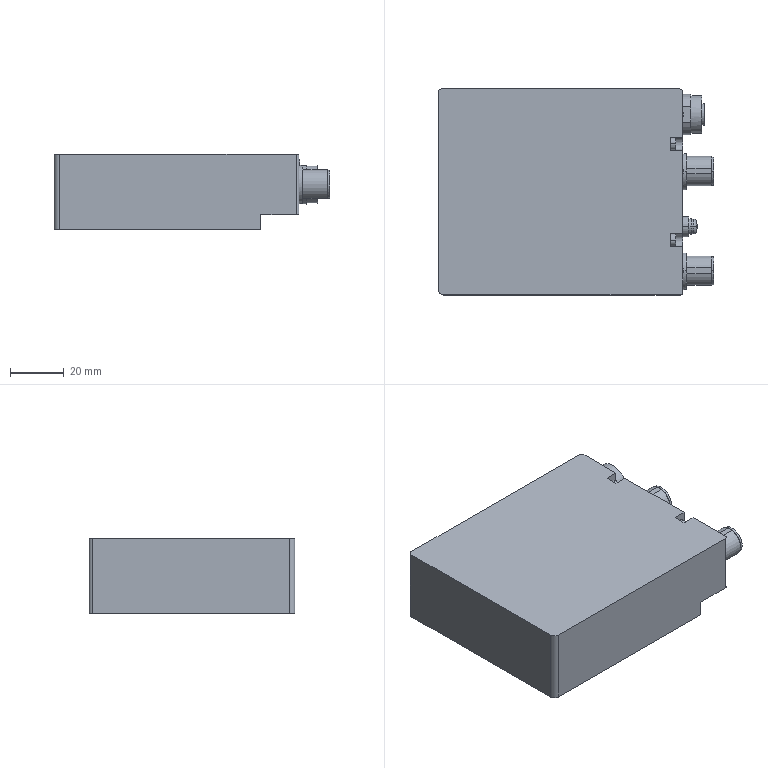Part | SolidWorks | features BaseBody 1 | 1 solid | 118 faces | box 102.4 x 76.5 x 28.2 mm | volume 193130 mm3 | plane 58 | cylinder 51 | cone 6 | spline 3 | commonest cylinder face diameters 4.5 x8 14 x8 4.7 x6 10.5 x4 10.9 x4 2.4 x3